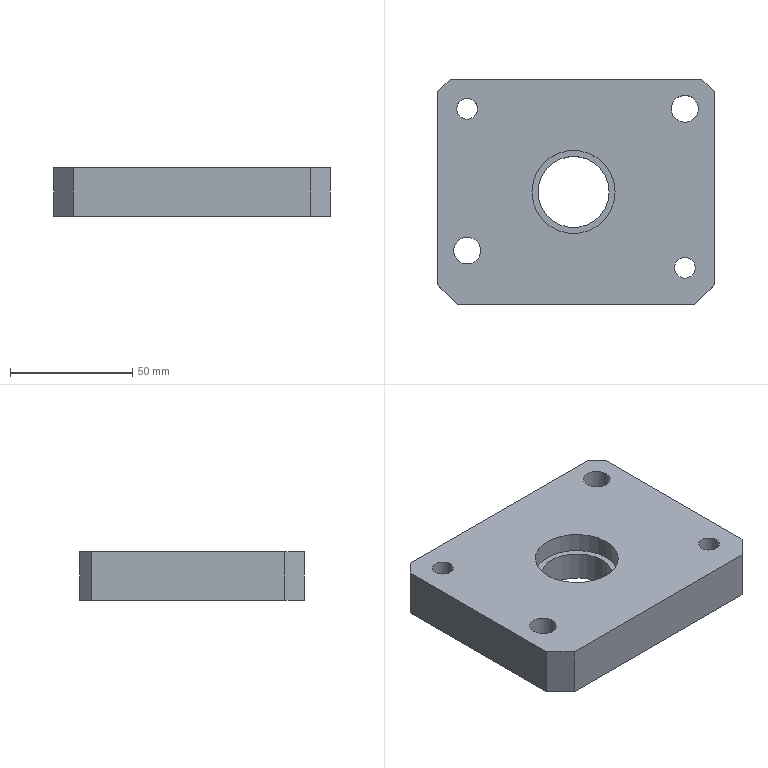Part | STEP file | lll_id3054_x_t | 1 solid | 26 faces | box 113 x 92 x 20 mm | volume 181138 mm3 | plane 15 | cylinder 11 | commonest cylinder face diameters 11 x4 8.5 x2 17 x2 29.07 x2 34 x1
STEP:
#1=CARTESIAN_POINT('',(3381.117,-235.288,22.5));
#2=VERTEX_POINT('',#1);
#3=CARTESIAN_POINT('',(3385.367,-235.288,22.5));
#4=DIRECTION('',(0.,0.,1.));
#5=DIRECTION('',(-1.,0.,0.));
#6=AXIS2_PLACEMENT_3D('',#3,#4,#5);
#7=CIRCLE('',#6,4.25);
#8=EDGE_CURVE('',#2,#2,#7,.T.);
#9=ORIENTED_EDGE('',*,*,#8,.F.);
#10=EDGE_LOOP('',(#9));
#11=FACE_BOUND('',#10,.T.);
#12=CARTESIAN_POINT('',(3292.117,-170.288,22.5));
#13=VERTEX_POINT('',#12);
#14=CARTESIAN_POINT('',(3296.367,-170.288,22.5));
#15=DIRECTION('',(0.,0.,1.));
#16=DIRECTION('',(-1.,0.,0.));
#17=AXIS2_PLACEMENT_3D('',#14,#15,#16);
#18=CIRCLE('',#17,4.25);
#19=EDGE_CURVE('',#13,#13,#18,.T.);
#20=ORIENTED_EDGE('',*,*,#19,.F.);
#21=EDGE_LOOP('',(#20));
#22=FACE_BOUND('',#21,.T.);
#23=CARTESIAN_POINT('',(3379.867,-170.288,22.5));
#24=VERTEX_POINT('',#23);
#25=CARTESIAN_POINT('',(3385.367,-170.288,22.5));
#26=DIRECTION('',(0.,0.,1.));
#27=DIRECTION('',(-1.,0.,0.));
#28=AXIS2_PLACEMENT_3D('',#25,#26,#27);
#29=CIRCLE('',#28,5.5);
#30=EDGE_CURVE('',#24,#24,#29,.T.);
#31=ORIENTED_EDGE('',*,*,#30,.F.);
#32=EDGE_LOOP('',(#31));
#33=FACE_BOUND('',#32,.T.);
#34=CARTESIAN_POINT('',(3389.367,-250.288,22.5));
#35=VERTEX_POINT('',#34);
#36=CARTESIAN_POINT('',(3292.367,-250.288,22.5));
#37=VERTEX_POINT('',#36);
#38=CARTESIAN_POINT('',(3341.867,-250.288,22.5));
#39=DIRECTION('',(-1.,0.,0.));
#40=VECTOR('',#39,1.);
#41=LINE('',#38,#40);
#42=EDGE_CURVE('',#35,#37,#41,.T.);
#43=ORIENTED_EDGE('',*,*,#42,.F.);
#44=CARTESIAN_POINT('',(3397.367,-242.288,22.5));
#45=VERTEX_POINT('',#44);
#46=CARTESIAN_POINT('',(3565.404,-74.251,22.5));
#47=DIRECTION('',(-0.7071,-0.7071,0.));
#48=VECTOR('',#47,1.);
#49=LINE('',#46,#48);
#50=EDGE_CURVE('',#45,#35,#49,.T.);
#51=ORIENTED_EDGE('',*,*,#50,.F.);
#52=CARTESIAN_POINT('',(3397.367,-163.288,22.5));
#53=VERTEX_POINT('',#52);
#54=CARTESIAN_POINT('',(3397.367,-195.288,22.5));
#55=DIRECTION('',(0.,-1.,0.));
#56=VECTOR('',#55,1.);
#57=LINE('',#54,#56);
#58=EDGE_CURVE('',#53,#45,#57,.T.);
#59=ORIENTED_EDGE('',*,*,#58,.F.);
#60=CARTESIAN_POINT('',(3392.367,-158.288,22.5));
#61=VERTEX_POINT('',#60);
#62=CARTESIAN_POINT('',(3528.747,-294.668,22.5));
#63=DIRECTION('',(0.7071,-0.7071,0.));
#64=VECTOR('',#63,1.);
#65=LINE('',#62,#64);
#66=EDGE_CURVE('',#61,#53,#65,.T.);
#67=ORIENTED_EDGE('',*,*,#66,.F.);
#68=CARTESIAN_POINT('',(3289.367,-158.288,22.5));
#69=VERTEX_POINT('',#68);
#70=CARTESIAN_POINT('',(3341.867,-158.288,22.5));
#71=DIRECTION('',(1.,0.,0.));
#72=VECTOR('',#71,1.);
#73=LINE('',#70,#72);
#74=EDGE_CURVE('',#69,#61,#73,.T.);
#75=ORIENTED_EDGE('',*,*,#74,.F.);
#76=CARTESIAN_POINT('',(3284.367,-163.288,22.5));
#77=VERTEX_POINT('',#76);
#78=CARTESIAN_POINT('',(3464.404,16.749,22.5));
#79=DIRECTION('',(0.7071,0.7071,0.));
#80=VECTOR('',#79,1.);
#81=LINE('',#78,#80);
#82=EDGE_CURVE('',#77,#69,#81,.T.);
#83=ORIENTED_EDGE('',*,*,#82,.F.);
#84=CARTESIAN_POINT('',(3284.367,-242.288,22.5));
#85=VERTEX_POINT('',#84);
#86=CARTESIAN_POINT('',(3284.367,-166.13,22.5));
#87=DIRECTION('',(0.,-1.,0.));
#88=VECTOR('',#87,1.);
#89=LINE('',#86,#88);
#90=EDGE_CURVE('',#77,#85,#89,.T.);
#91=ORIENTED_EDGE('',*,*,#90,.T.);
#92=CARTESIAN_POINT('',(3427.747,-385.668,22.5));
#93=DIRECTION('',(-0.7071,0.7071,0.));
#94=VECTOR('',#93,1.);
#95=LINE('',#92,#94);
#96=EDGE_CURVE('',#37,#85,#95,.T.);
#97=ORIENTED_EDGE('',*,*,#96,.F.);
#98=EDGE_LOOP('',(#43,#51,#59,#67,#75,#83,#91,#97));
#99=FACE_BOUND('',#98,.T.);
#100=CARTESIAN_POINT('',(3290.867,-228.288,22.5));
#101=VERTEX_POINT('',#100);
#102=CARTESIAN_POINT('',(3296.367,-228.288,22.5));
#103=DIRECTION('',(0.,0.,1.));
#104=DIRECTION('',(-1.,0.,0.));
#105=AXIS2_PLACEMENT_3D('',#102,#103,#104);
#106=CIRCLE('',#105,5.5);
#107=EDGE_CURVE('',#101,#101,#106,.T.);
#108=ORIENTED_EDGE('',*,*,#107,.F.);
#109=EDGE_LOOP('',(#108));
#110=FACE_BOUND('',#109,.T.);
#111=CARTESIAN_POINT('',(3356.867,-204.288,22.5));
#112=VERTEX_POINT('',#111);
#113=CARTESIAN_POINT('',(3339.867,-204.288,22.5));
#114=DIRECTION('',(0.,0.,-1.));
#115=DIRECTION('',(1.,0.,0.));
#116=AXIS2_PLACEMENT_3D('',#113,#114,#115);
#117=CIRCLE('',#116,17.);
#118=EDGE_CURVE('',#112,#112,#117,.T.);
#119=ORIENTED_EDGE('',*,*,#118,.T.);
#120=EDGE_LOOP('',(#119));
#121=FACE_BOUND('',#120,.T.);
#122=CARTESIAN_POINT('',(3651.284,-166.13,22.5));
#123=DIRECTION('',(0.,0.,1.));
#124=DIRECTION('',(0.,1.,0.));
#125=AXIS2_PLACEMENT_3D('',#122,#123,#124);
#126=PLANE('',#125);
#127=ADVANCED_FACE('',(#11,#22,#33,#99,#110,#121),#126,.T.);
#128=CARTESIAN_POINT('',(3354.402,-204.288,2.5));
#129=VERTEX_POINT('',#128);
#130=CARTESIAN_POINT('',(3325.332,-204.288,2.5));
#131=VERTEX_POINT('',#130);
#132=CARTESIAN_POINT('',(3339.867,-204.288,2.5));
#133=DIRECTION('',(0.,0.,-1.));
#134=DIRECTION('',(1.,0.,0.));
#135=AXIS2_PLACEMENT_3D('',#132,#133,#134);
#136=CIRCLE('',#135,14.535);
#137=EDGE_CURVE('',#129,#131,#136,.T.);
#138=ORIENTED_EDGE('',*,*,#137,.F.);
#139=CARTESIAN_POINT('',(3339.867,-204.288,2.5));
#140=DIRECTION('',(0.,0.,-1.));
#141=DIRECTION('',(1.,0.,0.));
#142=AXIS2_PLACEMENT_3D('',#139,#140,#141);
#143=CIRCLE('',#142,14.535);
#144=EDGE_CURVE('',#131,#129,#143,.T.);
#145=ORIENTED_EDGE('',*,*,#144,.F.);
#146=EDGE_LOOP('',(#138,#145));
#147=FACE_BOUND('',#146,.T.);
#148=CARTESIAN_POINT('',(3290.867,-170.288,2.5));
#149=VERTEX_POINT('',#148);
#150=CARTESIAN_POINT('',(3296.367,-170.288,2.5));
#151=DIRECTION('',(0.,0.,1.));
#152=DIRECTION('',(-1.,0.,0.));
#153=AXIS2_PLACEMENT_3D('',#150,#151,#152);
#154=CIRCLE('',#153,5.5);
#155=EDGE_CURVE('',#149,#149,#154,.T.);
#156=ORIENTED_EDGE('',*,*,#155,.T.);
#157=EDGE_LOOP('',(#156));
#158=FACE_BOUND('',#157,.T.);
#159=CARTESIAN_POINT('',(3376.867,-170.288,2.5));
#160=VERTEX_POINT('',#159);
#161=CARTESIAN_POINT('',(3385.367,-170.288,2.5));
#162=DIRECTION('',(0.,0.,-1.));
#163=DIRECTION('',(-1.,0.,0.));
#164=AXIS2_PLACEMENT_3D('',#161,#162,#163);
#165=CIRCLE('',#164,8.5);
#166=EDGE_CURVE('',#160,#160,#165,.T.);
#167=ORIENTED_EDGE('',*,*,#166,.F.);
#168=EDGE_LOOP('',(#167));
#169=FACE_BOUND('',#168,.T.);
#170=CARTESIAN_POINT('',(3284.367,-242.288,2.5));
#171=VERTEX_POINT('',#170);
#172=CARTESIAN_POINT('',(3284.367,-163.288,2.5));
#173=VERTEX_POINT('',#172);
#174=CARTESIAN_POINT('',(3284.367,-166.13,2.5));
#175=DIRECTION('',(0.,1.,0.));
#176=VECTOR('',#175,1.);
#177=LINE('',#174,#176);
#178=EDGE_CURVE('',#171,#173,#177,.T.);
#179=ORIENTED_EDGE('',*,*,#178,.T.);
#180=CARTESIAN_POINT('',(3289.367,-158.288,2.5));
#181=VERTEX_POINT('',#180);
#182=CARTESIAN_POINT('',(3464.404,16.749,2.5));
#183=DIRECTION('',(-0.7071,-0.7071,0.));
#184=VECTOR('',#183,1.);
#185=LINE('',#182,#184);
#186=EDGE_CURVE('',#181,#173,#185,.T.);
#187=ORIENTED_EDGE('',*,*,#186,.F.);
#188=CARTESIAN_POINT('',(3392.367,-158.288,2.5));
#189=VERTEX_POINT('',#188);
#190=CARTESIAN_POINT('',(3341.867,-158.288,2.5));
#191=DIRECTION('',(-1.,0.,0.));
#192=VECTOR('',#191,1.);
#193=LINE('',#190,#192);
#194=EDGE_CURVE('',#189,#181,#193,.T.);
#195=ORIENTED_EDGE('',*,*,#194,.F.);
#196=CARTESIAN_POINT('',(3397.367,-163.288,2.5));
#197=VERTEX_POINT('',#196);
#198=CARTESIAN_POINT('',(3528.747,-294.668,2.5));
#199=DIRECTION('',(-0.7071,0.7071,0.));
#200=VECTOR('',#199,1.);
#201=LINE('',#198,#200);
#202=EDGE_CURVE('',#197,#189,#201,.T.);
#203=ORIENTED_EDGE('',*,*,#202,.F.);
#204=CARTESIAN_POINT('',(3397.367,-242.288,2.5));
#205=VERTEX_POINT('',#204);
#206=CARTESIAN_POINT('',(3397.367,-195.288,2.5));
#207=DIRECTION('',(0.,1.,0.));
#208=VECTOR('',#207,1.);
#209=LINE('',#206,#208);
#210=EDGE_CURVE('',#205,#197,#209,.T.);
#211=ORIENTED_EDGE('',*,*,#210,.F.);
#212=CARTESIAN_POINT('',(3389.367,-250.288,2.5));
#213=VERTEX_POINT('',#212);
#214=CARTESIAN_POINT('',(3565.404,-74.251,2.5));
#215=DIRECTION('',(0.7071,0.7071,0.));
#216=VECTOR('',#215,1.);
#217=LINE('',#214,#216);
#218=EDGE_CURVE('',#213,#205,#217,.T.);
#219=ORIENTED_EDGE('',*,*,#218,.F.);
#220=CARTESIAN_POINT('',(3292.367,-250.288,2.5));
#221=VERTEX_POINT('',#220);
#222=CARTESIAN_POINT('',(3341.867,-250.288,2.5));
#223=DIRECTION('',(1.,0.,0.));
#224=VECTOR('',#223,1.);
#225=LINE('',#222,#224);
#226=EDGE_CURVE('',#221,#213,#225,.T.);
#227=ORIENTED_EDGE('',*,*,#226,.F.);
#228=CARTESIAN_POINT('',(3427.747,-385.668,2.5));
#229=DIRECTION('',(0.7071,-0.7071,0.));
#230=VECTOR('',#229,1.);
#231=LINE('',#228,#230);
#232=EDGE_CURVE('',#171,#221,#231,.T.);
#233=ORIENTED_EDGE('',*,*,#232,.F.);
#234=EDGE_LOOP('',(#179,#187,#195,#203,#211,#219,#227,#233));
#235=FACE_BOUND('',#234,.T.);
#236=CARTESIAN_POINT('',(3287.867,-228.288,2.5));
#237=VERTEX_POINT('',#236);
#238=CARTESIAN_POINT('',(3296.367,-228.288,2.5));
#239=DIRECTION('',(0.,0.,1.));
#240=DIRECTION('',(-1.,0.,0.));
#241=AXIS2_PLACEMENT_3D('',#238,#239,#240);
#242=CIRCLE('',#241,8.5);
#243=EDGE_CURVE('',#237,#237,#242,.T.);
#244=ORIENTED_EDGE('',*,*,#243,.T.);
#245=EDGE_LOOP('',(#244));
#246=FACE_BOUND('',#245,.T.);
#247=CARTESIAN_POINT('',(3379.867,-235.288,2.5));
#248=VERTEX_POINT('',#247);
#249=CARTESIAN_POINT('',(3385.367,-235.288,2.5));
#250=DIRECTION('',(0.,0.,-1.));
#251=DIRECTION('',(-1.,0.,0.));
#252=AXIS2_PLACEMENT_3D('',#249,#250,#251);
#253=CIRCLE('',#252,5.5);
#254=EDGE_CURVE('',#248,#248,#253,.T.);
#255=ORIENTED_EDGE('',*,*,#254,.F.);
#256=EDGE_LOOP('',(#255));
#257=FACE_BOUND('',#256,.T.);
#258=CARTESIAN_POINT('',(3651.284,-166.13,2.5));
#259=DIRECTION('',(0.,0.,1.));
#260=DIRECTION('',(0.,1.,0.));
#261=AXIS2_PLACEMENT_3D('',#258,#259,#260);
#262=PLANE('',#261);
#263=ADVANCED_FACE('',(#147,#158,#169,#235,#246,#257),#262,.F.);
#264=CARTESIAN_POINT('',(3292.117,-170.288,9.5));
#265=VERTEX_POINT('',#264);
#266=CARTESIAN_POINT('',(3296.367,-170.288,9.5));
#267=DIRECTION('',(0.,0.,-1.));
#268=DIRECTION('',(-1.,0.,0.));
#269=AXIS2_PLACEMENT_3D('',#266,#267,#268);
#270=CIRCLE('',#269,4.25);
#271=EDGE_CURVE('',#265,#265,#270,.T.);
#272=ORIENTED_EDGE('',*,*,#271,.F.);
#273=EDGE_LOOP('',(#272));
#274=FACE_BOUND('',#273,.T.);
#275=CARTESIAN_POINT('',(3290.867,-170.288,9.5));
#276=VERTEX_POINT('',#275);
#277=CARTESIAN_POINT('',(3296.367,-170.288,9.5));
#278=DIRECTION('',(0.,0.,-1.));
#279=DIRECTION('',(-1.,0.,0.));
#280=AXIS2_PLACEMENT_3D('',#277,#278,#279);
#281=CIRCLE('',#280,5.5);
#282=EDGE_CURVE('',#276,#276,#281,.T.);
#283=ORIENTED_EDGE('',*,*,#282,.T.);
#284=EDGE_LOOP('',(#283));
#285=FACE_BOUND('',#284,.T.);
#286=CARTESIAN_POINT('',(3296.367,-170.288,9.5));
#287=DIRECTION('',(0.,0.,1.));
#288=DIRECTION('',(-1.,0.,0.));
#289=AXIS2_PLACEMENT_3D('',#286,#287,#288);
#290=PLANE('',#289);
#291=ADVANCED_FACE('',(#274,#285),#290,.F.);
#292=CARTESIAN_POINT('',(3379.867,-170.288,14.5));
#293=VERTEX_POINT('',#292);
#294=CARTESIAN_POINT('',(3385.367,-170.288,14.5));
#295=DIRECTION('',(0.,0.,1.));
#296=DIRECTION('',(-1.,0.,0.));
#297=AXIS2_PLACEMENT_3D('',#294,#295,#296);
#298=CIRCLE('',#297,5.5);
#299=EDGE_CURVE('',#293,#293,#298,.T.);
#300=ORIENTED_EDGE('',*,*,#299,.T.);
#301=EDGE_LOOP('',(#300));
#302=FACE_BOUND('',#301,.T.);
#303=CARTESIAN_POINT('',(3376.867,-170.288,14.5));
#304=VERTEX_POINT('',#303);
#305=CARTESIAN_POINT('',(3385.367,-170.288,14.5));
#306=DIRECTION('',(0.,0.,1.));
#307=DIRECTION('',(-1.,0.,0.));
#308=AXIS2_PLACEMENT_3D('',#305,#306,#307);
#309=CIRCLE('',#308,8.5);
#310=EDGE_CURVE('',#304,#304,#309,.T.);
#311=ORIENTED_EDGE('',*,*,#310,.F.);
#312=EDGE_LOOP('',(#311));
#313=FACE_BOUND('',#312,.T.);
#314=CARTESIAN_POINT('',(3385.367,-170.288,14.5));
#315=DIRECTION('',(0.,0.,1.));
#316=DIRECTION('',(0.,-1.,0.));
#317=AXIS2_PLACEMENT_3D('',#314,#315,#316);
#318=PLANE('',#317);
#319=ADVANCED_FACE('',(#302,#313),#318,.F.);
#320=CARTESIAN_POINT('',(3290.867,-228.288,14.5));
#321=VERTEX_POINT('',#320);
#322=CARTESIAN_POINT('',(3296.367,-228.288,14.5));
#323=DIRECTION('',(0.,0.,-1.));
#324=DIRECTION('',(-1.,0.,0.));
#325=AXIS2_PLACEMENT_3D('',#322,#323,#324);
#326=CIRCLE('',#325,5.5);
#327=EDGE_CURVE('',#321,#321,#326,.T.);
#328=ORIENTED_EDGE('',*,*,#327,.F.);
#329=EDGE_LOOP('',(#328));
#330=FACE_BOUND('',#329,.T.);
#331=CARTESIAN_POINT('',(3287.867,-228.288,14.5));
#332=VERTEX_POINT('',#331);
#333=CARTESIAN_POINT('',(3296.367,-228.288,14.5));
#334=DIRECTION('',(0.,0.,-1.));
#335=DIRECTION('',(-1.,0.,0.));
#336=AXIS2_PLACEMENT_3D('',#333,#334,#335);
#337=CIRCLE('',#336,8.5);
#338=EDGE_CURVE('',#332,#332,#337,.T.);
#339=ORIENTED_EDGE('',*,*,#338,.T.);
#340=EDGE_LOOP('',(#339));
#341=FACE_BOUND('',#340,.T.);
#342=CARTESIAN_POINT('',(3296.367,-228.288,14.5));
#343=DIRECTION('',(0.,0.,1.));
#344=DIRECTION('',(0.,1.,0.));
#345=AXIS2_PLACEMENT_3D('',#342,#343,#344);
#346=PLANE('',#345);
#347=ADVANCED_FACE('',(#330,#341),#346,.F.);
#348=ORIENTED_EDGE('',*,*,#107,.T.);
#349=EDGE_LOOP('',(#348));
#350=FACE_BOUND('',#349,.T.);
#351=ORIENTED_EDGE('',*,*,#327,.T.);
#352=EDGE_LOOP('',(#351));
#353=FACE_BOUND('',#352,.T.);
#354=CARTESIAN_POINT('',(3296.367,-228.288,97.5));
#355=DIRECTION('',(0.,0.,1.));
#356=DIRECTION('',(0.,1.,0.));
#357=AXIS2_PLACEMENT_3D('',#354,#355,#356);
#358=CYLINDRICAL_SURFACE('',#357,5.5);
#359=ADVANCED_FACE('',(#350,#353),#358,.F.);
#360=ORIENTED_EDGE('',*,*,#282,.F.);
#361=EDGE_LOOP('',(#360));
#362=FACE_BOUND('',#361,.T.);
#363=ORIENTED_EDGE('',*,*,#155,.F.);
#364=EDGE_LOOP('',(#363));
#365=FACE_BOUND('',#364,.T.);
#366=CARTESIAN_POINT('',(3296.367,-170.288,-2.5));
#367=DIRECTION('',(0.,0.,1.));
#368=DIRECTION('',(-1.,0.,0.));
#369=AXIS2_PLACEMENT_3D('',#366,#367,#368);
#370=CYLINDRICAL_SURFACE('',#369,5.5);
#371=ADVANCED_FACE('',(#362,#365),#370,.F.);
#372=ORIENTED_EDGE('',*,*,#310,.T.);
#373=EDGE_LOOP('',(#372));
#374=FACE_BOUND('',#373,.T.);
#375=ORIENTED_EDGE('',*,*,#166,.T.);
#376=EDGE_LOOP('',(#375));
#377=FACE_BOUND('',#376,.T.);
#378=CARTESIAN_POINT('',(3385.367,-170.288,-2.5));
#379=DIRECTION('',(0.,0.,1.));
#380=DIRECTION('',(0.,-1.,0.));
#381=AXIS2_PLACEMENT_3D('',#378,#379,#380);
#382=CYLINDRICAL_SURFACE('',#381,8.5);
#383=ADVANCED_FACE('',(#374,#377),#382,.F.);
#384=ORIENTED_EDGE('',*,*,#210,.T.);
#385=CARTESIAN_POINT('',(3397.367,-163.288,-81.5));
#386=DIRECTION('',(0.,0.,-1.));
#387=VECTOR('',#386,1.);
#388=LINE('',#385,#387);
#389=EDGE_CURVE('',#53,#197,#388,.T.);
#390=ORIENTED_EDGE('',*,*,#389,.F.);
#391=ORIENTED_EDGE('',*,*,#58,.T.);
#392=CARTESIAN_POINT('',(3397.367,-242.288,-81.5));
#393=DIRECTION('',(0.,0.,1.));
#394=VECTOR('',#393,1.);
#395=LINE('',#392,#394);
#396=EDGE_CURVE('',#205,#45,#395,.T.);
#397=ORIENTED_EDGE('',*,*,#396,.F.);
#398=EDGE_LOOP('',(#384,#390,#391,#397));
#399=FACE_OUTER_BOUND('',#398,.T.);
#400=CARTESIAN_POINT('',(3397.367,-195.288,-81.5));
#401=DIRECTION('',(1.,0.,0.));
#402=DIRECTION('',(0.,0.,-1.));
#403=AXIS2_PLACEMENT_3D('',#400,#401,#402);
#404=PLANE('',#403);
#405=ADVANCED_FACE('',(#399),#404,.T.);
#406=ORIENTED_EDGE('',*,*,#194,.T.);
#407=CARTESIAN_POINT('',(3289.367,-158.288,-81.5));
#408=DIRECTION('',(0.,0.,-1.));
#409=VECTOR('',#408,1.);
#410=LINE('',#407,#409);
#411=EDGE_CURVE('',#69,#181,#410,.T.);
#412=ORIENTED_EDGE('',*,*,#411,.F.);
#413=ORIENTED_EDGE('',*,*,#74,.T.);
#414=CARTESIAN_POINT('',(3392.367,-158.288,-81.5));
#415=DIRECTION('',(0.,0.,1.));
#416=VECTOR('',#415,1.);
#417=LINE('',#414,#416);
#418=EDGE_CURVE('',#189,#61,#417,.T.);
#419=ORIENTED_EDGE('',*,*,#418,.F.);
#420=EDGE_LOOP('',(#406,#412,#413,#419));
#421=FACE_OUTER_BOUND('',#420,.T.);
#422=CARTESIAN_POINT('',(3341.867,-158.288,-81.5));
#423=DIRECTION('',(0.,1.,0.));
#424=DIRECTION('',(0.,0.,-1.));
#425=AXIS2_PLACEMENT_3D('',#422,#423,#424);
#426=PLANE('',#425);
#427=ADVANCED_FACE('',(#421),#426,.T.);
#428=ORIENTED_EDGE('',*,*,#90,.F.);
#429=CARTESIAN_POINT('',(3284.367,-163.288,13.5));
#430=DIRECTION('',(0.,0.,1.));
#431=VECTOR('',#430,1.);
#432=LINE('',#429,#431);
#433=EDGE_CURVE('',#173,#77,#432,.T.);
#434=ORIENTED_EDGE('',*,*,#433,.F.);
#435=ORIENTED_EDGE('',*,*,#178,.F.);
#436=CARTESIAN_POINT('',(3284.367,-242.288,13.5));
#437=DIRECTION('',(0.,0.,-1.));
#438=VECTOR('',#437,1.);
#439=LINE('',#436,#438);
#440=EDGE_CURVE('',#85,#171,#439,.T.);
#441=ORIENTED_EDGE('',*,*,#440,.F.);
#442=EDGE_LOOP('',(#428,#434,#435,#441));
#443=FACE_OUTER_BOUND('',#442,.T.);
#444=CARTESIAN_POINT('',(3284.367,-195.288,13.5));
#445=DIRECTION('',(-1.,0.,0.));
#446=DIRECTION('',(0.,0.,1.));
#447=AXIS2_PLACEMENT_3D('',#444,#445,#446);
#448=PLANE('',#447);
#449=ADVANCED_FACE('',(#443),#448,.T.);
#450=ORIENTED_EDGE('',*,*,#226,.T.);
#451=CARTESIAN_POINT('',(3389.367,-250.288,-81.5));
#452=DIRECTION('',(0.,0.,-1.));
#453=VECTOR('',#452,1.);
#454=LINE('',#451,#453);
#455=EDGE_CURVE('',#35,#213,#454,.T.);
#456=ORIENTED_EDGE('',*,*,#455,.F.);
#457=ORIENTED_EDGE('',*,*,#42,.T.);
#458=CARTESIAN_POINT('',(3292.367,-250.288,-81.5));
#459=DIRECTION('',(0.,0.,1.));
#460=VECTOR('',#459,1.);
#461=LINE('',#458,#460);
#462=EDGE_CURVE('',#221,#37,#461,.T.);
#463=ORIENTED_EDGE('',*,*,#462,.F.);
#464=EDGE_LOOP('',(#450,#456,#457,#463));
#465=FACE_OUTER_BOUND('',#464,.T.);
#466=CARTESIAN_POINT('',(3341.867,-250.288,-81.5));
#467=DIRECTION('',(0.,-1.,0.));
#468=DIRECTION('',(0.,0.,1.));
#469=AXIS2_PLACEMENT_3D('',#466,#467,#468);
#470=PLANE('',#469);
#471=ADVANCED_FACE('',(#465),#470,.T.);
#472=ORIENTED_EDGE('',*,*,#338,.F.);
#473=EDGE_LOOP('',(#472));
#474=FACE_BOUND('',#473,.T.);
#475=ORIENTED_EDGE('',*,*,#243,.F.);
#476=EDGE_LOOP('',(#475));
#477=FACE_BOUND('',#476,.T.);
#478=CARTESIAN_POINT('',(3296.367,-228.288,-2.5));
#479=DIRECTION('',(0.,0.,1.));
#480=DIRECTION('',(0.,1.,0.));
#481=AXIS2_PLACEMENT_3D('',#478,#479,#480);
#482=CYLINDRICAL_SURFACE('',#481,8.5);
#483=ADVANCED_FACE('',(#474,#477),#482,.F.);
#484=ORIENTED_EDGE('',*,*,#30,.T.);
#485=EDGE_LOOP('',(#484));
#486=FACE_BOUND('',#485,.T.);
#487=ORIENTED_EDGE('',*,*,#299,.F.);
#488=EDGE_LOOP('',(#487));
#489=FACE_BOUND('',#488,.T.);
#490=CARTESIAN_POINT('',(3385.367,-170.288,97.5));
#491=DIRECTION('',(0.,0.,1.));
#492=DIRECTION('',(0.,-1.,0.));
#493=AXIS2_PLACEMENT_3D('',#490,#491,#492);
#494=CYLINDRICAL_SURFACE('',#493,5.5);
#495=ADVANCED_FACE('',(#486,#489),#494,.F.);
#496=ORIENTED_EDGE('',*,*,#19,.T.);
#497=EDGE_LOOP('',(#496));
#498=FACE_BOUND('',#497,.T.);
#499=ORIENTED_EDGE('',*,*,#271,.T.);
#500=EDGE_LOOP('',(#499));
#501=FACE_BOUND('',#500,.T.);
#502=CARTESIAN_POINT('',(3296.367,-170.288,97.5));
#503=DIRECTION('',(0.,0.,1.));
#504=DIRECTION('',(-1.,0.,0.));
#505=AXIS2_PLACEMENT_3D('',#502,#503,#504);
#506=CYLINDRICAL_SURFACE('',#505,4.25);
#507=ADVANCED_FACE('',(#498,#501),#506,.F.);
#508=ORIENTED_EDGE('',*,*,#8,.T.);
#509=EDGE_LOOP('',(#508));
#510=FACE_BOUND('',#509,.T.);
#511=CARTESIAN_POINT('',(3381.117,-235.288,9.5));
#512=VERTEX_POINT('',#511);
#513=CARTESIAN_POINT('',(3385.367,-235.288,9.5));
#514=DIRECTION('',(0.,0.,-1.));
#515=DIRECTION('',(-1.,0.,0.));
#516=AXIS2_PLACEMENT_3D('',#513,#514,#515);
#517=CIRCLE('',#516,4.25);
#518=EDGE_CURVE('',#512,#512,#517,.T.);
#519=ORIENTED_EDGE('',*,*,#518,.T.);
#520=EDGE_LOOP('',(#519));
#521=FACE_BOUND('',#520,.T.);
#522=CARTESIAN_POINT('',(3385.367,-235.288,97.5));
#523=DIRECTION('',(0.,0.,1.));
#524=DIRECTION('',(1.,0.,0.));
#525=AXIS2_PLACEMENT_3D('',#522,#523,#524);
#526=CYLINDRICAL_SURFACE('',#525,4.25);
#527=ADVANCED_FACE('',(#510,#521),#526,.F.);
#528=ORIENTED_EDGE('',*,*,#518,.F.);
#529=EDGE_LOOP('',(#528));
#530=FACE_BOUND('',#529,.T.);
#531=CARTESIAN_POINT('',(3379.867,-235.288,9.5));
#532=VERTEX_POINT('',#531);
#533=CARTESIAN_POINT('',(3385.367,-235.288,9.5));
#534=DIRECTION('',(0.,0.,-1.));
#535=DIRECTION('',(-1.,0.,0.));
#536=AXIS2_PLACEMENT_3D('',#533,#534,#535);
#537=CIRCLE('',#536,5.5);
#538=EDGE_CURVE('',#532,#532,#537,.T.);
#539=ORIENTED_EDGE('',*,*,#538,.T.);
#540=EDGE_LOOP('',(#539));
#541=FACE_BOUND('',#540,.T.);
#542=CARTESIAN_POINT('',(3385.367,-235.288,9.5));
#543=DIRECTION('',(0.,0.,1.));
#544=DIRECTION('',(1.,0.,0.));
#545=AXIS2_PLACEMENT_3D('',#542,#543,#544);
#546=PLANE('',#545);
#547=ADVANCED_FACE('',(#530,#541),#546,.F.);
#548=ORIENTED_EDGE('',*,*,#538,.F.);
#549=EDGE_LOOP('',(#548));
#550=FACE_BOUND('',#549,.T.);
#551=ORIENTED_EDGE('',*,*,#254,.T.);
#552=EDGE_LOOP('',(#551));
#553=FACE_BOUND('',#552,.T.);
#554=CARTESIAN_POINT('',(3385.367,-235.288,-2.5));
#555=DIRECTION('',(0.,0.,1.));
#556=DIRECTION('',(1.,0.,0.));
#557=AXIS2_PLACEMENT_3D('',#554,#555,#556);
#558=CYLINDRICAL_SURFACE('',#557,5.5);
#559=ADVANCED_FACE('',(#550,#553),#558,.F.);
#560=ORIENTED_EDGE('',*,*,#66,.T.);
#561=ORIENTED_EDGE('',*,*,#389,.T.);
#562=ORIENTED_EDGE('',*,*,#202,.T.);
#563=ORIENTED_EDGE('',*,*,#418,.T.);
#564=EDGE_LOOP('',(#560,#561,#562,#563));
#565=FACE_OUTER_BOUND('',#564,.T.);
#566=CARTESIAN_POINT('',(3397.367,-163.288,-81.5));
#567=DIRECTION('',(-0.7071,-0.7071,0.));
#568=DIRECTION('',(0.,0.,-1.));
#569=AXIS2_PLACEMENT_3D('',#566,#567,#568);
#570=PLANE('',#569);
#571=ADVANCED_FACE('',(#565),#570,.F.);
#572=ORIENTED_EDGE('',*,*,#82,.T.);
#573=ORIENTED_EDGE('',*,*,#411,.T.);
#574=ORIENTED_EDGE('',*,*,#186,.T.);
#575=ORIENTED_EDGE('',*,*,#433,.T.);
#576=EDGE_LOOP('',(#572,#573,#574,#575));
#577=FACE_OUTER_BOUND('',#576,.T.);
#578=CARTESIAN_POINT('',(3289.367,-158.288,-81.5));
#579=DIRECTION('',(0.7071,-0.7071,0.));
#580=DIRECTION('',(0.,0.,-1.));
#581=AXIS2_PLACEMENT_3D('',#578,#579,#580);
#582=PLANE('',#581);
#583=ADVANCED_FACE('',(#577),#582,.F.);
#584=ORIENTED_EDGE('',*,*,#232,.T.);
#585=ORIENTED_EDGE('',*,*,#462,.T.);
#586=ORIENTED_EDGE('',*,*,#96,.T.);
#587=ORIENTED_EDGE('',*,*,#440,.T.);
#588=EDGE_LOOP('',(#584,#585,#586,#587));
#589=FACE_OUTER_BOUND('',#588,.T.);
#590=CARTESIAN_POINT('',(3292.367,-250.288,-81.5));
#591=DIRECTION('',(0.7071,0.7071,0.));
#592=DIRECTION('',(0.,0.,1.));
#593=AXIS2_PLACEMENT_3D('',#590,#591,#592);
#594=PLANE('',#593);
#595=ADVANCED_FACE('',(#589),#594,.F.);
#596=ORIENTED_EDGE('',*,*,#50,.T.);
#597=ORIENTED_EDGE('',*,*,#455,.T.);
#598=ORIENTED_EDGE('',*,*,#218,.T.);
#599=ORIENTED_EDGE('',*,*,#396,.T.);
#600=EDGE_LOOP('',(#596,#597,#598,#599));
#601=FACE_OUTER_BOUND('',#600,.T.);
#602=CARTESIAN_POINT('',(3389.367,-250.288,-81.5));
#603=DIRECTION('',(-0.7071,0.7071,0.));
#604=DIRECTION('',(0.,0.,-1.));
#605=AXIS2_PLACEMENT_3D('',#602,#603,#604);
#606=PLANE('',#605);
#607=ADVANCED_FACE('',(#601),#606,.F.);
#608=CARTESIAN_POINT('',(3325.332,-204.288,14.5));
#609=VERTEX_POINT('',#608);
#610=CARTESIAN_POINT('',(3325.332,-204.288,5.));
#611=DIRECTION('',(0.,0.,-1.));
#612=VECTOR('',#611,1.);
#613=LINE('',#610,#612);
#614=EDGE_CURVE('',#609,#131,#613,.T.);
#615=ORIENTED_EDGE('',*,*,#614,.F.);
#616=CARTESIAN_POINT('',(3354.402,-204.288,14.5));
#617=VERTEX_POINT('',#616);
#618=CARTESIAN_POINT('',(3339.867,-204.288,14.5));
#619=DIRECTION('',(0.,0.,1.));
#620=DIRECTION('',(-1.,0.,0.));
#621=AXIS2_PLACEMENT_3D('',#618,#619,#620);
#622=CIRCLE('',#621,14.535);
#623=EDGE_CURVE('',#609,#617,#622,.T.);
#624=ORIENTED_EDGE('',*,*,#623,.T.);
#625=CARTESIAN_POINT('',(3354.402,-204.288,5.));
#626=DIRECTION('',(0.,0.,1.));
#627=VECTOR('',#626,1.);
#628=LINE('',#625,#627);
#629=EDGE_CURVE('',#129,#617,#628,.T.);
#630=ORIENTED_EDGE('',*,*,#629,.F.);
#631=ORIENTED_EDGE('',*,*,#137,.T.);
#632=EDGE_LOOP('',(#615,#624,#630,#631));
#633=FACE_OUTER_BOUND('',#632,.T.);
#634=CARTESIAN_POINT('',(3339.867,-204.288,5.));
#635=DIRECTION('',(0.,0.,-1.));
#636=DIRECTION('',(-1.,0.,0.));
#637=AXIS2_PLACEMENT_3D('',#634,#635,#636);
#638=CYLINDRICAL_SURFACE('',#637,14.535);
#639=ADVANCED_FACE('',(#633),#638,.F.);
#640=ORIENTED_EDGE('',*,*,#629,.T.);
#641=CARTESIAN_POINT('',(3339.867,-204.288,14.5));
#642=DIRECTION('',(0.,0.,1.));
#643=DIRECTION('',(-1.,0.,0.));
#644=AXIS2_PLACEMENT_3D('',#641,#642,#643);
#645=CIRCLE('',#644,14.535);
#646=EDGE_CURVE('',#617,#609,#645,.T.);
#647=ORIENTED_EDGE('',*,*,#646,.T.);
#648=ORIENTED_EDGE('',*,*,#614,.T.);
#649=ORIENTED_EDGE('',*,*,#144,.T.);
#650=EDGE_LOOP('',(#640,#647,#648,#649));
#651=FACE_OUTER_BOUND('',#650,.T.);
#652=CARTESIAN_POINT('',(3339.867,-204.288,5.));
#653=DIRECTION('',(0.,0.,-1.));
#654=DIRECTION('',(-1.,0.,0.));
#655=AXIS2_PLACEMENT_3D('',#652,#653,#654);
#656=CYLINDRICAL_SURFACE('',#655,14.535);
#657=ADVANCED_FACE('',(#651),#656,.F.);
#658=CARTESIAN_POINT('',(3322.867,-204.288,14.5));
#659=VERTEX_POINT('',#658);
#660=CARTESIAN_POINT('',(3339.867,-204.288,14.5));
#661=DIRECTION('',(0.,0.,1.));
#662=DIRECTION('',(-1.,0.,0.));
#663=AXIS2_PLACEMENT_3D('',#660,#661,#662);
#664=CIRCLE('',#663,17.);
#665=EDGE_CURVE('',#659,#659,#664,.T.);
#666=ORIENTED_EDGE('',*,*,#665,.T.);
#667=EDGE_LOOP('',(#666));
#668=FACE_BOUND('',#667,.T.);
#669=ORIENTED_EDGE('',*,*,#646,.F.);
#670=ORIENTED_EDGE('',*,*,#623,.F.);
#671=EDGE_LOOP('',(#669,#670));
#672=FACE_BOUND('',#671,.T.);
#673=CARTESIAN_POINT('',(3339.867,-204.288,14.5));
#674=DIRECTION('',(0.,0.,-1.));
#675=DIRECTION('',(-1.,0.,0.));
#676=AXIS2_PLACEMENT_3D('',#673,#674,#675);
#677=PLANE('',#676);
#678=ADVANCED_FACE('',(#668,#672),#677,.F.);
#679=ORIENTED_EDGE('',*,*,#118,.F.);
#680=EDGE_LOOP('',(#679));
#681=FACE_BOUND('',#680,.T.);
#682=ORIENTED_EDGE('',*,*,#665,.F.);
#683=EDGE_LOOP('',(#682));
#684=FACE_BOUND('',#683,.T.);
#685=CARTESIAN_POINT('',(3339.867,-204.288,14.5));
#686=DIRECTION('',(0.,0.,1.));
#687=DIRECTION('',(1.,0.,0.));
#688=AXIS2_PLACEMENT_3D('',#685,#686,#687);
#689=CYLINDRICAL_SURFACE('',#688,17.);
#690=ADVANCED_FACE('',(#681,#684),#689,.F.);
#691=CLOSED_SHELL('',(#127,#263,#291,#319,#347,#359,#371,#383,#405,#427,#449,#471,#483,#495,#507,#527,#547,#559,#571,#583,#595,#607,#639,#657,#678,#690));
#692=MANIFOLD_SOLID_BREP('',#691);
#693=(LENGTH_UNIT()NAMED_UNIT(*)SI_UNIT(.MILLI.,.METRE.));
#694=UNCERTAINTY_MEASURE_WITH_UNIT(LENGTH_MEASURE(0.00002),#693,'','');
#695=(NAMED_UNIT(*)PLANE_ANGLE_UNIT()SI_UNIT($,.RADIAN.));
#696=PLANE_ANGLE_MEASURE_WITH_UNIT(PLANE_ANGLE_MEASURE(0.01745),#695);
#697=DIMENSIONAL_EXPONENTS(0.,0.,0.,0.,0.,0.,0.);
#698=(CONVERSION_BASED_UNIT('DEGREE',#696)NAMED_UNIT(#697)PLANE_ANGLE_UNIT());
#699=(NAMED_UNIT(*)SI_UNIT($,.STERADIAN.)SOLID_ANGLE_UNIT());
#700=(GEOMETRIC_REPRESENTATION_CONTEXT(3)GLOBAL_UNCERTAINTY_ASSIGNED_CONTEXT((#694))GLOBAL_UNIT_ASSIGNED_CONTEXT((#693,#698,#699))REPRESENTATION_CONTEXT('',''));
#701=ADVANCED_BREP_SHAPE_REPRESENTATION('',(#692),#700);